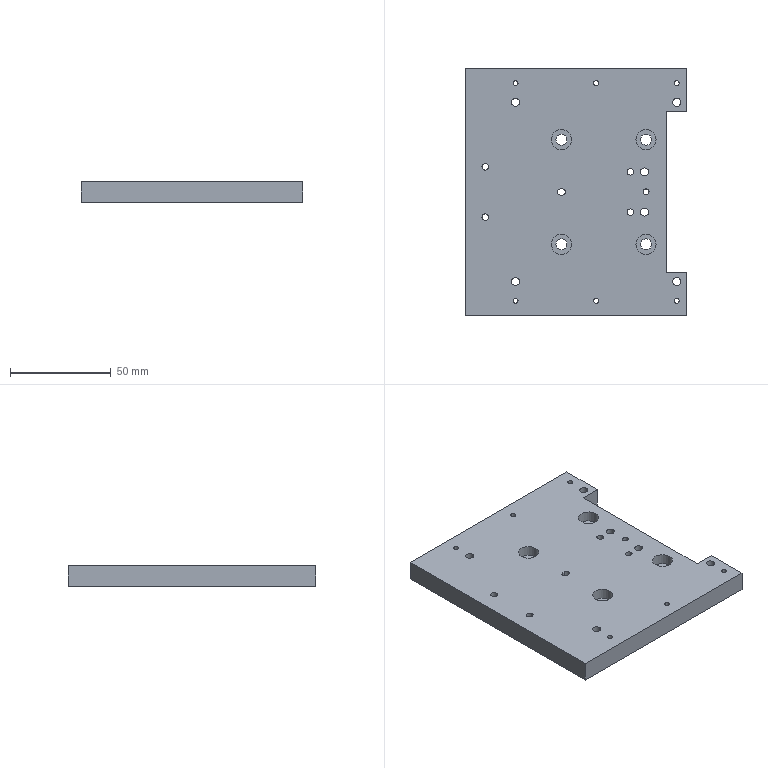CAM job | NX | 3-axis milling, drilling | part box 110 x 123 x 10 mm | stock box 115 x 130 x 12 mm
Tools:
number,name,description,diameter,corner_radius,flute_length,length,flutes
6,D6,平底铣刀-粗,6.0,0.0,25.0,75.0,2
9,D10,平底铣刀-粗,10.0,0.0,35.0,75.0,2
11,D2-J,平底铣刀-精,2.0,0.0,50.0,75.0,2
7,D6-J,平底铣刀-精,6.0,0.0,25.0,75.0,2
1,D80R0.8飞刀,圆鼻刀-粗,80.0,0.8,50.0,75.0,2
1,D80R0.8飞刀-J,圆鼻刀-精,80.0,0.8,50.0,75.0,2
2,D6倒角刀,倒角刀,6.0,0.0,3.0,25.0,2
20,M3X0.5,丝锥,2.5,0.0,35.0,50.0,2
21,M4X0.7,丝锥,3.3,0.0,35.0,50.0,2
22,D3铰刀,Drilling Tool,3.0,0.0,75.0,100.0,6
23,D4铰刀,Drilling Tool,4.0,0.0,75.0,100.0,6
12,ZT2.6,钻头,2.6,0.0,35.0,50.0,2
13,ZT3.4,钻头,3.4,0.0,35.0,50.0,2
19,ZT5.5,钻头,5.5,0.0,35.0,50.0,2
17,ZT2.9,Drilling Tool,2.9,0.0,35.0,50.0,2
18,ZT3.9,Drilling Tool,3.9,0.0,35.0,50.0,2
Operations:
program,operation,operation_type,tool,method,geometry_group,spindle_rpm,surface_speed,feed_per_tooth,feed_cut,feed_plunge,cut_length_mm,path_length_mm,cut_time_min,machine_time_min
B,底壁铣飞面开粗_COPY,VolumeBased25DMillingOperation,D80R0.8飞刀,分层开粗-切深K-步距G,W-B,2800.0,703.696,0.5357,3000.0,100.0,1929.416,2188.298,0.6431,0.669
B,底壁铣飞面精光_COPY,VolumeBased25DMillingOperation,D80R0.8飞刀-J,侧刃精光-切深K-步距G,W-B,4000.0,1005.28,0.125,1000.0,100.0,481.767,577.766,0.4818,0.4914
B,NG_钻倒角_5,Operation,D6倒角刀,METHOD,W-B,8000.0,150.796,0.0625,1000.0,0.0,28.5,440.491,0.0285,0.0697
B,NG_钻倒角_6,Operation,D6倒角刀,METHOD,W-B,8000.0,150.796,0.0625,1000.0,0.0,4.8,109.6,0.0048,0.0153
B,NG_钻倒角_7,Operation,D6倒角刀,METHOD,W-B,8000.0,150.796,0.0625,1000.0,0.0,31.8,435.232,0.0318,0.0721
B,NG_钻倒角_8,Operation,D6倒角刀,METHOD,W-B,8000.0,150.796,0.0625,1000.0,0.0,20.8,268.109,0.0208,0.0455
B,铣倒角_2,PlanarMilling,D6倒角刀,METHOD,W-B,8000.0,150.796,0.075,1200.0,100.0,71.178,615.712,0.0593,0.1138
B,平面去毛刺6X45L_COPY,SurfaceContour,D6倒角刀,爬面_倒角-切深0-步距G,W-B,6500.0,122.519,0.1154,1500.0,100.0,664.892,1477.922,0.4433,0.5246
A,顶面,FaceMilling,D80R0.8飞刀,侧刃精光-切深K-步距G,W-A,4500.0,1385.0,0.1667,1500.0,100.0,718.0,814.0,0.4787,0.4883
A,动态开粗D10_COPY,CavityMilling,D10,动态开粗-切深K-步距K,W-A,8000.0,251.32,0.25,4000.0,100.0,4890.978,5006.978,1.223,1.234
A,打点-深0.8,Operation,D6倒角刀,NONE,W-A,8000.0,150.796,0.0312,500.0,90.0,37.8,623.348,0.0756,0.1342
A,打点-深0.8_COPY,Operation,D6倒角刀,NONE,W-A,8000.0,150.796,0.0312,500.0,90.0,1.8,103.6,0.0036,0.0138
A,通孔-M3螺纹底孔,Operation,ZT2.6,NONE,W-A,3000.0,23.562,0.05,300.0,90.0,102.0,577.055,0.34,0.3875
A,通孔-精孔3.0预钻,Operation,ZT2.9,NONE,W-A,3200.0,29.154,0.0312,200.0,90.0,14.837,129.674,0.0742,0.0857
A,通孔-精孔3.0预钻_COPY,Operation,ZT2.9,NONE,W-A,3200.0,29.154,0.0312,200.0,90.0,14.837,129.674,0.0742,0.0857
A,通孔-M4螺纹底孔,Operation,ZT3.4,NONE,W-A,3000.0,31.102,0.05,300.0,90.0,68.0,356.095,0.2267,0.2555
A,通孔-精孔4.0预钻,Operation,ZT3.9,NONE,W-A,3000.0,36.757,0.0417,250.0,90.0,90.755,542.633,0.363,0.4082
A,沉头孔-钻孔0段,Operation,ZT5.5,NONE,W-A,1200.0,20.735,0.0625,150.0,90.0,58.609,356.252,0.3907,0.4205
A,通腰槽粗_1,VolumeBased25DMillingOperation,D2-J,METHOD,W-A,12000.0,75.398,0.0167,400.0,100.0,513.317,621.817,1.283,1.294
A,等高光顺清角D2参考6_COPY,ZLevelMilling,D2-J,分层精光-切深K-步距G,W-A,12000.0,75.398,0.0625,1500.0,100.0,1347.2,1542.501,0.8981,0.9177
A,铣孔开粗D6_1,CylinderMilling,D6,NONE,W-A,8000.0,150.796,0.075,1200.0,100.0,635.598,1191.198,0.5297,0.5852
A,铣孔精光D6_1,CylinderMilling,D6-J,精光步距切深关,W-A,8000.0,150.796,0.0312,500.0,100.0,133.594,691.194,0.2672,0.3229
A,仅选体,SurfaceContour,D6倒角刀,METHOD,W-A,8000.0,150.796,0.1875,3000.0,100.0,515.297,754.969,0.1718,0.1957
A,NG_钻倒角_1,Operation,D6倒角刀,METHOD,W-A,8000.0,150.796,0.0312,500.0,0.0,28.5,440.491,0.057,0.0982
A,NG_钻倒角_2,Operation,D6倒角刀,METHOD,W-A,8000.0,150.796,0.0312,500.0,0.0,4.8,109.6,0.0096,0.0201
A,NG_钻倒角_3,Operation,D6倒角刀,METHOD,W-A,8000.0,150.796,0.0312,500.0,0.0,20.8,268.109,0.0416,0.0663
A,NG_钻倒角_4,Operation,D6倒角刀,METHOD,W-A,8000.0,150.796,0.0312,500.0,0.0,31.8,435.232,0.0636,0.1039
A,铣倒角_1,PlanarMilling,D6倒角刀,NONE,W-A,8000.0,150.796,0.05,800.0,100.0,161.004,685.685,0.2013,0.2537
A,腰槽精_1,VolumeBased25DMillingOperation,D2-J,METHOD,W-A,8000.0,50.266,0.0125,200.0,100.0,37.529,176.034,0.1876,0.2015
A,REAMING,Operation,D3铰刀,METHOD,W-A,500.0,4.712,0.0167,50.0,0.0,12.0,124.0,0.24,0.2512
A,REAMING_2,Operation,D4铰刀,METHOD,W-A,500.0,6.283,0.0167,50.0,0.0,72.0,505.123,1.44,1.483
A,通孔-攻牙M3,Operation,M3X0.5,METHOD,W-A,800.0,6.283,0.0003,0.5,90.0,84.0,541.055,168.0,168.046
A,通孔-攻牙M4,Operation,M4X0.7,METHOD,W-A,600.0,6.22,0.0006,0.7,90.0,56.0,332.095,80.0,80.028
A,外形半精_2,VolumeBased25DMillingOperation,D6-J,METHOD,W-A,9000.0,169.646,0.0667,1200.0,100.0,507.191,626.191,0.4227,0.4346